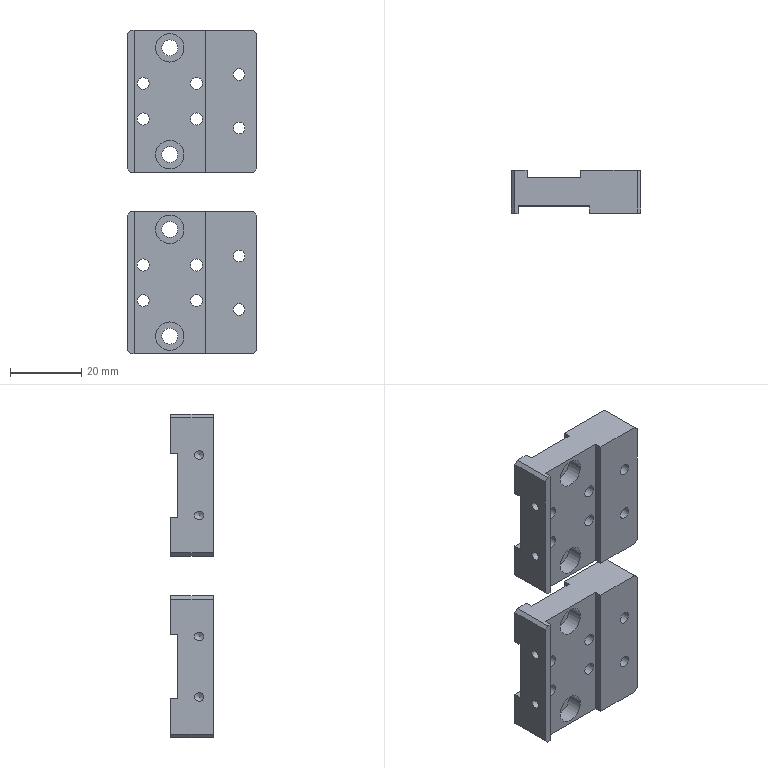Part | 2 solids | 124 faces | box 36.5 x 12 x 91 mm | volume 22154 mm3 | plane 72 | cylinder 44 | cone 8 | commonest cylinder face diameters 2.5 x8 3.4 x8 6.5 x8 2 x4 3.3 x4 4 x4